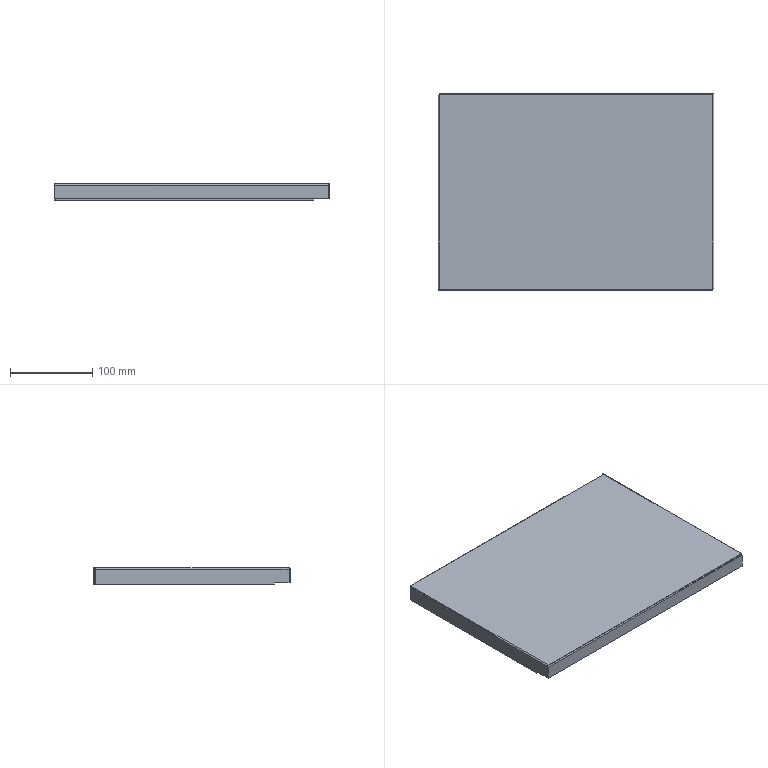Part | SolidWorks | features BaseBody 1 | 1 solid | 44 faces | box 336 x 239.8 x 20 mm | volume 120306 mm3 | plane 32 | cylinder 8 | spline 4 | commonest cylinder face diameters 1 x4 3.4 x4
STEP:
#1=CARTESIAN_POINT('',(-168.,-118.2,-18.));
#2=VERTEX_POINT('',#1);
#3=CARTESIAN_POINT('',(-168.,-100.2,-18.));
#4=VERTEX_POINT('',#3);
#5=CARTESIAN_POINT('',(-168.,-118.2,-18.));
#6=DIRECTION('',(0.,1.,0.));
#7=VECTOR('',#6,1000.);
#8=LINE('',#5,#7);
#9=EDGE_CURVE('',#2,#4,#8,.T.);
#10=ORIENTED_EDGE('',*,*,#9,.T.);
#11=CARTESIAN_POINT('',(-166.8,-100.2,-18.));
#12=VERTEX_POINT('',#11);
#13=CARTESIAN_POINT('',(-166.8,-100.2,-18.));
#14=DIRECTION('',(-1.,0.,0.));
#15=VECTOR('',#14,1000.);
#16=LINE('',#13,#15);
#17=EDGE_CURVE('',#12,#4,#16,.T.);
#18=ORIENTED_EDGE('',*,*,#17,.F.);
#19=CARTESIAN_POINT('',(-166.8,-118.2,-18.));
#20=VERTEX_POINT('',#19);
#21=CARTESIAN_POINT('',(-166.8,-118.2,-18.));
#22=DIRECTION('',(0.,1.,0.));
#23=VECTOR('',#22,1000.);
#24=LINE('',#21,#23);
#25=EDGE_CURVE('',#20,#12,#24,.T.);
#26=ORIENTED_EDGE('',*,*,#25,.F.);
#27=CARTESIAN_POINT('',(-166.8,-118.2,-18.));
#28=DIRECTION('',(-1.,0.,0.));
#29=VECTOR('',#28,1000.);
#30=LINE('',#27,#29);
#31=EDGE_CURVE('',#20,#2,#30,.T.);
#32=ORIENTED_EDGE('',*,*,#31,.T.);
#33=EDGE_LOOP('',(#10,#18,#26,#32));
#34=FACE_OUTER_BOUND('',#33,.T.);
#35=CARTESIAN_POINT('',(-166.8,-118.2,-18.));
#36=DIRECTION('',(0.,0.,1.));
#37=DIRECTION('',(1.,0.,0.));
#38=AXIS2_PLACEMENT_3D('',#35,#36,#37);
#39=PLANE('',#38);
#40=ADVANCED_FACE('',(#34),#39,.F.);
#41=CARTESIAN_POINT('',(-168.,-100.2,-20.));
#42=VERTEX_POINT('',#41);
#43=CARTESIAN_POINT('',(-168.,-100.2,-20.));
#44=DIRECTION('',(0.,0.,-1.));
#45=VECTOR('',#44,1000.);
#46=LINE('',#43,#45);
#47=EDGE_CURVE('',#4,#42,#46,.T.);
#48=ORIENTED_EDGE('',*,*,#47,.T.);
#49=CARTESIAN_POINT('',(-166.8,-100.2,-20.));
#50=VERTEX_POINT('',#49);
#51=CARTESIAN_POINT('',(-166.8,-100.2,-20.));
#52=DIRECTION('',(-1.,0.,0.));
#53=VECTOR('',#52,1000.);
#54=LINE('',#51,#53);
#55=EDGE_CURVE('',#50,#42,#54,.T.);
#56=ORIENTED_EDGE('',*,*,#55,.F.);
#57=CARTESIAN_POINT('',(-166.8,-100.2,-20.));
#58=DIRECTION('',(0.,0.,-1.));
#59=VECTOR('',#58,1000.);
#60=LINE('',#57,#59);
#61=EDGE_CURVE('',#12,#50,#60,.T.);
#62=ORIENTED_EDGE('',*,*,#61,.F.);
#63=ORIENTED_EDGE('',*,*,#17,.T.);
#64=EDGE_LOOP('',(#48,#56,#62,#63));
#65=FACE_OUTER_BOUND('',#64,.T.);
#66=CARTESIAN_POINT('',(-166.8,-100.2,-20.));
#67=DIRECTION('',(0.,1.,0.));
#68=DIRECTION('',(1.,0.,0.));
#69=AXIS2_PLACEMENT_3D('',#66,#67,#68);
#70=PLANE('',#69);
#71=ADVANCED_FACE('',(#65),#70,.F.);
#72=CARTESIAN_POINT('',(148.3,119.9,-20.));
#73=VERTEX_POINT('',#72);
#74=CARTESIAN_POINT('',(148.3,119.9,-18.));
#75=VERTEX_POINT('',#74);
#76=CARTESIAN_POINT('',(148.3,119.9,-20.));
#77=DIRECTION('',(0.,0.,1.));
#78=VECTOR('',#77,1000.);
#79=LINE('',#76,#78);
#80=EDGE_CURVE('',#73,#75,#79,.T.);
#81=ORIENTED_EDGE('',*,*,#80,.T.);
#82=CARTESIAN_POINT('',(148.3,118.7,-18.));
#83=VERTEX_POINT('',#82);
#84=CARTESIAN_POINT('',(148.3,118.7,-18.));
#85=DIRECTION('',(0.,1.,0.));
#86=VECTOR('',#85,1000.);
#87=LINE('',#84,#86);
#88=EDGE_CURVE('',#83,#75,#87,.T.);
#89=ORIENTED_EDGE('',*,*,#88,.F.);
#90=CARTESIAN_POINT('',(148.3,118.7,-20.));
#91=VERTEX_POINT('',#90);
#92=CARTESIAN_POINT('',(148.3,118.7,-20.));
#93=DIRECTION('',(0.,0.,1.));
#94=VECTOR('',#93,1000.);
#95=LINE('',#92,#94);
#96=EDGE_CURVE('',#91,#83,#95,.T.);
#97=ORIENTED_EDGE('',*,*,#96,.F.);
#98=CARTESIAN_POINT('',(148.3,118.7,-20.));
#99=DIRECTION('',(0.,1.,0.));
#100=VECTOR('',#99,1000.);
#101=LINE('',#98,#100);
#102=EDGE_CURVE('',#91,#73,#101,.T.);
#103=ORIENTED_EDGE('',*,*,#102,.T.);
#104=EDGE_LOOP('',(#81,#89,#97,#103));
#105=FACE_OUTER_BOUND('',#104,.T.);
#106=CARTESIAN_POINT('',(148.3,118.7,-20.));
#107=DIRECTION('',(-1.,0.,0.));
#108=DIRECTION('',(0.,1.,0.));
#109=AXIS2_PLACEMENT_3D('',#106,#107,#108);
#110=PLANE('',#109);
#111=ADVANCED_FACE('',(#105),#110,.F.);
#112=CARTESIAN_POINT('',(166.3,119.9,-18.));
#113=VERTEX_POINT('',#112);
#114=CARTESIAN_POINT('',(166.3,119.9,-18.));
#115=DIRECTION('',(1.,0.,0.));
#116=VECTOR('',#115,1000.);
#117=LINE('',#114,#116);
#118=EDGE_CURVE('',#75,#113,#117,.T.);
#119=ORIENTED_EDGE('',*,*,#118,.T.);
#120=CARTESIAN_POINT('',(166.3,118.7,-18.));
#121=VERTEX_POINT('',#120);
#122=CARTESIAN_POINT('',(166.3,118.7,-18.));
#123=DIRECTION('',(0.,1.,0.));
#124=VECTOR('',#123,1000.);
#125=LINE('',#122,#124);
#126=EDGE_CURVE('',#121,#113,#125,.T.);
#127=ORIENTED_EDGE('',*,*,#126,.F.);
#128=CARTESIAN_POINT('',(166.3,118.7,-18.));
#129=DIRECTION('',(1.,0.,0.));
#130=VECTOR('',#129,1000.);
#131=LINE('',#128,#130);
#132=EDGE_CURVE('',#83,#121,#131,.T.);
#133=ORIENTED_EDGE('',*,*,#132,.F.);
#134=ORIENTED_EDGE('',*,*,#88,.T.);
#135=EDGE_LOOP('',(#119,#127,#133,#134));
#136=FACE_OUTER_BOUND('',#135,.T.);
#137=CARTESIAN_POINT('',(166.3,118.7,-18.));
#138=DIRECTION('',(0.,0.,1.));
#139=DIRECTION('',(0.,-1.,0.));
#140=AXIS2_PLACEMENT_3D('',#137,#138,#139);
#141=PLANE('',#140);
#142=ADVANCED_FACE('',(#136),#141,.F.);
#143=CARTESIAN_POINT('',(166.3,118.7,-1.7));
#144=VERTEX_POINT('',#143);
#145=CARTESIAN_POINT('',(166.3,118.7,-20.));
#146=DIRECTION('',(0.,0.,-1.));
#147=VECTOR('',#146,1000.);
#148=LINE('',#145,#147);
#149=EDGE_CURVE('',#144,#121,#148,.T.);
#150=ORIENTED_EDGE('',*,*,#149,.T.);
#151=ORIENTED_EDGE('',*,*,#126,.T.);
#152=CARTESIAN_POINT('',(166.3,119.9,-1.7));
#153=VERTEX_POINT('',#152);
#154=CARTESIAN_POINT('',(166.3,119.9,0.));
#155=DIRECTION('',(0.,0.,-1.));
#156=VECTOR('',#155,1000.);
#157=LINE('',#154,#156);
#158=EDGE_CURVE('',#153,#113,#157,.T.);
#159=ORIENTED_EDGE('',*,*,#158,.F.);
#160=CARTESIAN_POINT('',(166.3,118.7,-1.7));
#161=DIRECTION('',(0.,1.,0.));
#162=VECTOR('',#161,1000.);
#163=LINE('',#160,#162);
#164=EDGE_CURVE('',#144,#153,#163,.T.);
#165=ORIENTED_EDGE('',*,*,#164,.F.);
#166=EDGE_LOOP('',(#150,#151,#159,#165));
#167=FACE_OUTER_BOUND('',#166,.T.);
#168=CARTESIAN_POINT('',(166.3,119.9,-20.));
#169=DIRECTION('',(-1.,0.,0.));
#170=DIRECTION('',(0.,1.,0.));
#171=AXIS2_PLACEMENT_3D('',#168,#169,#170);
#172=PLANE('',#171);
#173=ADVANCED_FACE('',(#167),#172,.F.);
#174=CARTESIAN_POINT('',(-166.093,119.9,-20.));
#175=VERTEX_POINT('',#174);
#176=CARTESIAN_POINT('',(0.,119.9,-20.));
#177=DIRECTION('',(-1.,0.,0.));
#178=VECTOR('',#177,1000.);
#179=LINE('',#176,#178);
#180=EDGE_CURVE('',#73,#175,#179,.T.);
#181=ORIENTED_EDGE('',*,*,#180,.F.);
#182=ORIENTED_EDGE('',*,*,#102,.F.);
#183=CARTESIAN_POINT('',(-166.093,118.7,-20.));
#184=VERTEX_POINT('',#183);
#185=CARTESIAN_POINT('',(-168.,118.7,-20.));
#186=DIRECTION('',(-1.,0.,0.));
#187=VECTOR('',#186,1000.);
#188=LINE('',#185,#187);
#189=EDGE_CURVE('',#91,#184,#188,.T.);
#190=ORIENTED_EDGE('',*,*,#189,.T.);
#191=CARTESIAN_POINT('',(-166.093,118.7,-20.));
#192=DIRECTION('',(0.,-1.,0.));
#193=VECTOR('',#192,1000.);
#194=LINE('',#191,#193);
#195=EDGE_CURVE('',#175,#184,#194,.T.);
#196=ORIENTED_EDGE('',*,*,#195,.F.);
#197=EDGE_LOOP('',(#181,#182,#190,#196));
#198=FACE_OUTER_BOUND('',#197,.T.);
#199=CARTESIAN_POINT('',(-168.,119.9,-20.));
#200=DIRECTION('',(0.,0.,1.));
#201=DIRECTION('',(0.,-1.,0.));
#202=AXIS2_PLACEMENT_3D('',#199,#200,#201);
#203=PLANE('',#202);
#204=ADVANCED_FACE('',(#198),#203,.F.);
#205=ORIENTED_EDGE('',*,*,#132,.T.);
#206=ORIENTED_EDGE('',*,*,#149,.F.);
#207=CARTESIAN_POINT('',(-166.093,118.7,-1.7));
#208=VERTEX_POINT('',#207);
#209=CARTESIAN_POINT('',(-168.,118.7,-1.7));
#210=DIRECTION('',(1.,0.,0.));
#211=VECTOR('',#210,1000.);
#212=LINE('',#209,#211);
#213=EDGE_CURVE('',#208,#144,#212,.T.);
#214=ORIENTED_EDGE('',*,*,#213,.F.);
#215=CARTESIAN_POINT('',(-166.093,118.7,0.));
#216=DIRECTION('',(0.,0.,-1.));
#217=VECTOR('',#216,1000.);
#218=LINE('',#215,#217);
#219=EDGE_CURVE('',#208,#184,#218,.T.);
#220=ORIENTED_EDGE('',*,*,#219,.T.);
#221=ORIENTED_EDGE('',*,*,#189,.F.);
#222=ORIENTED_EDGE('',*,*,#96,.T.);
#223=EDGE_LOOP('',(#205,#206,#214,#220,#221,#222));
#224=FACE_OUTER_BOUND('',#223,.T.);
#225=CARTESIAN_POINT('',(0.,118.7,0.));
#226=DIRECTION('',(0.,-1.,0.));
#227=DIRECTION('',(0.,0.,-1.));
#228=AXIS2_PLACEMENT_3D('',#225,#226,#227);
#229=PLANE('',#228);
#230=ADVANCED_FACE('',(#224),#229,.T.);
#231=ORIENTED_EDGE('',*,*,#158,.T.);
#232=ORIENTED_EDGE('',*,*,#118,.F.);
#233=ORIENTED_EDGE('',*,*,#80,.F.);
#234=ORIENTED_EDGE('',*,*,#180,.T.);
#235=CARTESIAN_POINT('',(-166.093,119.9,-1.7));
#236=VERTEX_POINT('',#235);
#237=CARTESIAN_POINT('',(-166.093,119.9,-1.2));
#238=DIRECTION('',(0.,0.,-1.));
#239=VECTOR('',#238,1000.);
#240=LINE('',#237,#239);
#241=EDGE_CURVE('',#236,#175,#240,.T.);
#242=ORIENTED_EDGE('',*,*,#241,.F.);
#243=CARTESIAN_POINT('',(-168.,119.9,-1.7));
#244=DIRECTION('',(-1.,0.,0.));
#245=VECTOR('',#244,1000.);
#246=LINE('',#243,#245);
#247=EDGE_CURVE('',#153,#236,#246,.T.);
#248=ORIENTED_EDGE('',*,*,#247,.F.);
#249=EDGE_LOOP('',(#231,#232,#233,#234,#242,#248));
#250=FACE_OUTER_BOUND('',#249,.T.);
#251=CARTESIAN_POINT('',(0.,119.9,0.));
#252=DIRECTION('',(0.,-1.,0.));
#253=DIRECTION('',(0.,0.,-1.));
#254=AXIS2_PLACEMENT_3D('',#251,#252,#253);
#255=PLANE('',#254);
#256=ADVANCED_FACE('',(#250),#255,.F.);
#257=ORIENTED_EDGE('',*,*,#241,.T.);
#258=ORIENTED_EDGE('',*,*,#195,.T.);
#259=ORIENTED_EDGE('',*,*,#219,.F.);
#260=CARTESIAN_POINT('',(-166.093,118.7,-1.7));
#261=DIRECTION('',(0.,-1.,0.));
#262=VECTOR('',#261,1000.);
#263=LINE('',#260,#262);
#264=EDGE_CURVE('',#236,#208,#263,.T.);
#265=ORIENTED_EDGE('',*,*,#264,.F.);
#266=EDGE_LOOP('',(#257,#258,#259,#265));
#267=FACE_OUTER_BOUND('',#266,.T.);
#268=CARTESIAN_POINT('',(-166.093,118.7,-1.2));
#269=DIRECTION('',(-1.,0.,0.));
#270=DIRECTION('',(0.,0.,1.));
#271=AXIS2_PLACEMENT_3D('',#268,#269,#270);
#272=PLANE('',#271);
#273=ADVANCED_FACE('',(#267),#272,.T.);
#274=CARTESIAN_POINT('',(166.3,118.2,-1.2));
#275=VERTEX_POINT('',#274);
#276=CARTESIAN_POINT('',(-166.3,118.2,-1.2));
#277=VERTEX_POINT('',#276);
#278=CARTESIAN_POINT('',(166.3,118.2,-1.2));
#279=DIRECTION('',(-1.,0.,0.));
#280=VECTOR('',#279,1000.);
#281=LINE('',#278,#280);
#282=EDGE_CURVE('',#275,#277,#281,.T.);
#283=ORIENTED_EDGE('',*,*,#282,.T.);
#284=CARTESIAN_POINT('',(-166.3,118.2,-1.2));
#285=CARTESIAN_POINT('',(-166.265,118.331,-1.2));
#286=CARTESIAN_POINT('',(-166.231,118.461,-1.254));
#287=CARTESIAN_POINT('',(-166.162,118.646,-1.439));
#288=CARTESIAN_POINT('',(-166.127,118.7,-1.569));
#289=CARTESIAN_POINT('',(-166.093,118.7,-1.7));
#290=B_SPLINE_CURVE_WITH_KNOTS('',3,(#284,#285,#286,#287,#288,#289),.UNSPECIFIED.,.F.,.F.,(4,2,4),(0.,0.5,1.),.UNSPECIFIED.);
#291=EDGE_CURVE('',#277,#208,#290,.T.);
#292=ORIENTED_EDGE('',*,*,#291,.T.);
#293=ORIENTED_EDGE('',*,*,#213,.T.);
#294=CARTESIAN_POINT('',(166.3,118.2,-1.7));
#295=DIRECTION('',(1.,0.,0.));
#296=DIRECTION('',(0.,0.,-1.));
#297=AXIS2_PLACEMENT_3D('',#294,#295,#296);
#298=CIRCLE('',#297,0.5);
#299=EDGE_CURVE('',#144,#275,#298,.T.);
#300=ORIENTED_EDGE('',*,*,#299,.T.);
#301=EDGE_LOOP('',(#283,#292,#293,#300));
#302=FACE_OUTER_BOUND('',#301,.T.);
#303=CARTESIAN_POINT('',(166.3,118.2,-1.7));
#304=DIRECTION('',(1.,0.,0.));
#305=DIRECTION('',(0.,1.,0.));
#306=AXIS2_PLACEMENT_3D('',#303,#304,#305);
#307=CYLINDRICAL_SURFACE('',#306,0.5);
#308=ADVANCED_FACE('',(#302),#307,.F.);
#309=CARTESIAN_POINT('',(166.3,118.2,0.));
#310=VERTEX_POINT('',#309);
#311=CARTESIAN_POINT('',(-166.3,118.2,0.));
#312=VERTEX_POINT('',#311);
#313=CARTESIAN_POINT('',(166.3,118.2,0.));
#314=DIRECTION('',(-1.,0.,0.));
#315=VECTOR('',#314,1000.);
#316=LINE('',#313,#315);
#317=EDGE_CURVE('',#310,#312,#316,.T.);
#318=ORIENTED_EDGE('',*,*,#317,.F.);
#319=CARTESIAN_POINT('',(166.3,119.825,-1.2));
#320=VERTEX_POINT('',#319);
#321=CARTESIAN_POINT('',(166.3,118.2,-1.7));
#322=DIRECTION('',(1.,0.,0.));
#323=DIRECTION('',(0.,0.,-1.));
#324=AXIS2_PLACEMENT_3D('',#321,#322,#323);
#325=CIRCLE('',#324,1.7);
#326=EDGE_CURVE('',#320,#310,#325,.T.);
#327=ORIENTED_EDGE('',*,*,#326,.F.);
#328=CARTESIAN_POINT('',(166.3,118.2,-1.7));
#329=DIRECTION('',(1.,0.,0.));
#330=DIRECTION('',(0.,0.,-1.));
#331=AXIS2_PLACEMENT_3D('',#328,#329,#330);
#332=CIRCLE('',#331,1.7);
#333=EDGE_CURVE('',#153,#320,#332,.T.);
#334=ORIENTED_EDGE('',*,*,#333,.F.);
#335=ORIENTED_EDGE('',*,*,#247,.T.);
#336=CARTESIAN_POINT('',(-166.3,118.2,0.));
#337=CARTESIAN_POINT('',(-166.283,118.423,0.));
#338=CARTESIAN_POINT('',(-166.265,118.645,-0.04425));
#339=CARTESIAN_POINT('',(-166.231,119.056,-0.2146));
#340=CARTESIAN_POINT('',(-166.214,119.245,-0.3406));
#341=CARTESIAN_POINT('',(-166.179,119.559,-0.6553));
#342=CARTESIAN_POINT('',(-166.162,119.685,-0.8438));
#343=CARTESIAN_POINT('',(-166.127,119.856,-1.255));
#344=CARTESIAN_POINT('',(-166.11,119.9,-1.477));
#345=CARTESIAN_POINT('',(-166.093,119.9,-1.7));
#346=B_SPLINE_CURVE_WITH_KNOTS('',3,(#336,#337,#338,#339,#340,#341,#342,#343,#344,#345),.UNSPECIFIED.,.F.,.F.,(4,2,2,2,4),(0.,0.25,0.5,0.75,1.),.UNSPECIFIED.);
#347=EDGE_CURVE('',#312,#236,#346,.T.);
#348=ORIENTED_EDGE('',*,*,#347,.F.);
#349=EDGE_LOOP('',(#318,#327,#334,#335,#348));
#350=FACE_OUTER_BOUND('',#349,.T.);
#351=CARTESIAN_POINT('',(166.3,118.2,-1.7));
#352=DIRECTION('',(1.,0.,0.));
#353=DIRECTION('',(0.,1.,0.));
#354=AXIS2_PLACEMENT_3D('',#351,#352,#353);
#355=CYLINDRICAL_SURFACE('',#354,1.7);
#356=ADVANCED_FACE('',(#350),#355,.T.);
#357=ORIENTED_EDGE('',*,*,#333,.T.);
#358=CARTESIAN_POINT('',(166.3,119.9,-1.2));
#359=DIRECTION('',(0.,-1.,0.));
#360=VECTOR('',#359,1000.);
#361=LINE('',#358,#360);
#362=EDGE_CURVE('',#320,#275,#361,.T.);
#363=ORIENTED_EDGE('',*,*,#362,.T.);
#364=ORIENTED_EDGE('',*,*,#299,.F.);
#365=ORIENTED_EDGE('',*,*,#164,.T.);
#366=EDGE_LOOP('',(#357,#363,#364,#365));
#367=FACE_OUTER_BOUND('',#366,.T.);
#368=CARTESIAN_POINT('',(166.3,118.2,-1.7));
#369=DIRECTION('',(-1.,0.,0.));
#370=DIRECTION('',(0.,1.,0.));
#371=AXIS2_PLACEMENT_3D('',#368,#369,#370);
#372=PLANE('',#371);
#373=ADVANCED_FACE('',(#367),#372,.F.);
#374=ORIENTED_EDGE('',*,*,#264,.T.);
#375=ORIENTED_EDGE('',*,*,#291,.F.);
#376=CARTESIAN_POINT('',(-166.3,118.2,-1.2));
#377=DIRECTION('',(0.,0.,1.));
#378=VECTOR('',#377,1000.);
#379=LINE('',#376,#378);
#380=EDGE_CURVE('',#277,#312,#379,.T.);
#381=ORIENTED_EDGE('',*,*,#380,.T.);
#382=ORIENTED_EDGE('',*,*,#347,.T.);
#383=EDGE_LOOP('',(#374,#375,#381,#382));
#384=FACE_OUTER_BOUND('',#383,.T.);
#385=CARTESIAN_POINT('',(-166.3,118.2,0.012));
#386=CARTESIAN_POINT('',(-166.283,118.424,0.012));
#387=CARTESIAN_POINT('',(-166.265,118.648,-0.03256));
#388=CARTESIAN_POINT('',(-166.231,119.062,-0.2041));
#389=CARTESIAN_POINT('',(-166.214,119.252,-0.331));
#390=CARTESIAN_POINT('',(-166.179,119.569,-0.6479));
#391=CARTESIAN_POINT('',(-166.162,119.696,-0.8378));
#392=CARTESIAN_POINT('',(-166.127,119.867,-1.252));
#393=CARTESIAN_POINT('',(-166.11,119.912,-1.476));
#394=CARTESIAN_POINT('',(-166.093,119.912,-1.7));
#395=CARTESIAN_POINT('',(-166.3,118.2,0.));
#396=CARTESIAN_POINT('',(-166.283,118.423,0.));
#397=CARTESIAN_POINT('',(-166.265,118.645,-0.04425));
#398=CARTESIAN_POINT('',(-166.231,119.056,-0.2146));
#399=CARTESIAN_POINT('',(-166.214,119.245,-0.3406));
#400=CARTESIAN_POINT('',(-166.179,119.559,-0.6553));
#401=CARTESIAN_POINT('',(-166.162,119.685,-0.8438));
#402=CARTESIAN_POINT('',(-166.127,119.856,-1.255));
#403=CARTESIAN_POINT('',(-166.11,119.9,-1.477));
#404=CARTESIAN_POINT('',(-166.093,119.9,-1.7));
#405=CARTESIAN_POINT('',(-166.3,118.2,-1.2));
#406=CARTESIAN_POINT('',(-166.283,118.265,-1.2));
#407=CARTESIAN_POINT('',(-166.265,118.331,-1.213));
#408=CARTESIAN_POINT('',(-166.231,118.452,-1.263));
#409=CARTESIAN_POINT('',(-166.214,118.507,-1.3));
#410=CARTESIAN_POINT('',(-166.179,118.6,-1.393));
#411=CARTESIAN_POINT('',(-166.162,118.637,-1.448));
#412=CARTESIAN_POINT('',(-166.127,118.687,-1.569));
#413=CARTESIAN_POINT('',(-166.11,118.7,-1.635));
#414=CARTESIAN_POINT('',(-166.093,118.7,-1.7));
#415=CARTESIAN_POINT('',(-166.3,118.2,-1.212));
#416=CARTESIAN_POINT('',(-166.283,118.264,-1.212));
#417=CARTESIAN_POINT('',(-166.265,118.328,-1.225));
#418=CARTESIAN_POINT('',(-166.231,118.446,-1.274));
#419=CARTESIAN_POINT('',(-166.214,118.5,-1.31));
#420=CARTESIAN_POINT('',(-166.179,118.59,-1.4));
#421=CARTESIAN_POINT('',(-166.162,118.626,-1.454));
#422=CARTESIAN_POINT('',(-166.127,118.675,-1.572));
#423=CARTESIAN_POINT('',(-166.11,118.688,-1.636));
#424=CARTESIAN_POINT('',(-166.093,118.688,-1.7));
#425=B_SPLINE_SURFACE_WITH_KNOTS('',1,3,((#385,#386,#387,#388,#389,#390,#391,#392,#393,#394),(#395,#396,#397,#398,#399,#400,#401,#402,#403,#404),(#405,#406,#407,#408,#409,#410,#411,#412,#413,#414),(#415,#416,#417,#418,#419,#420,#421,#422,#423,#424)),.UNSPECIFIED.,.F.,.F.,.F.,(2,1,1,2),(4,2,2,2,4),(-0.01,0.,1.,1.01),(0.,0.25,0.5,0.75,1.),.UNSPECIFIED.);
#426=ADVANCED_FACE('',(#384),#425,.F.);
#427=CARTESIAN_POINT('',(-168.,117.993,-20.));
#428=VERTEX_POINT('',#427);
#429=CARTESIAN_POINT('',(-166.8,117.993,-20.));
#430=VERTEX_POINT('',#429);
#431=CARTESIAN_POINT('',(-168.,117.993,-20.));
#432=DIRECTION('',(1.,0.,0.));
#433=VECTOR('',#432,1000.);
#434=LINE('',#431,#433);
#435=EDGE_CURVE('',#428,#430,#434,.T.);
#436=ORIENTED_EDGE('',*,*,#435,.F.);
#437=CARTESIAN_POINT('',(-168.,117.993,-1.7));
#438=VERTEX_POINT('',#437);
#439=CARTESIAN_POINT('',(-168.,117.993,0.));
#440=DIRECTION('',(0.,0.,-1.));
#441=VECTOR('',#440,1000.);
#442=LINE('',#439,#441);
#443=EDGE_CURVE('',#438,#428,#442,.T.);
#444=ORIENTED_EDGE('',*,*,#443,.F.);
#445=CARTESIAN_POINT('',(-166.8,117.993,-1.7));
#446=VERTEX_POINT('',#445);
#447=CARTESIAN_POINT('',(-166.8,117.993,-1.7));
#448=DIRECTION('',(1.,0.,0.));
#449=VECTOR('',#448,1000.);
#450=LINE('',#447,#449);
#451=EDGE_CURVE('',#438,#446,#450,.T.);
#452=ORIENTED_EDGE('',*,*,#451,.T.);
#453=CARTESIAN_POINT('',(-166.8,117.993,-1.2));
#454=DIRECTION('',(0.,0.,-1.));
#455=VECTOR('',#454,1000.);
#456=LINE('',#453,#455);
#457=EDGE_CURVE('',#446,#430,#456,.T.);
#458=ORIENTED_EDGE('',*,*,#457,.T.);
#459=EDGE_LOOP('',(#436,#444,#452,#458));
#460=FACE_OUTER_BOUND('',#459,.T.);
#461=CARTESIAN_POINT('',(-166.8,117.993,-1.2));
#462=DIRECTION('',(0.,-1.,0.));
#463=DIRECTION('',(0.,0.,-1.));
#464=AXIS2_PLACEMENT_3D('',#461,#462,#463);
#465=PLANE('',#464);
#466=ADVANCED_FACE('',(#460),#465,.F.);
#467=CARTESIAN_POINT('',(-166.8,-118.2,-20.));
#468=DIRECTION('',(0.,-1.,0.));
#469=VECTOR('',#468,1000.);
#470=LINE('',#467,#469);
#471=EDGE_CURVE('',#430,#50,#470,.T.);
#472=ORIENTED_EDGE('',*,*,#471,.T.);
#473=ORIENTED_EDGE('',*,*,#55,.T.);
#474=CARTESIAN_POINT('',(-168.,0.,-20.));
#475=DIRECTION('',(0.,-1.,0.));
#476=VECTOR('',#475,1000.);
#477=LINE('',#474,#476);
#478=EDGE_CURVE('',#428,#42,#477,.T.);
#479=ORIENTED_EDGE('',*,*,#478,.F.);
#480=ORIENTED_EDGE('',*,*,#435,.T.);
#481=EDGE_LOOP('',(#472,#473,#479,#480));
#482=FACE_OUTER_BOUND('',#481,.T.);
#483=CARTESIAN_POINT('',(-168.,-118.2,-20.));
#484=DIRECTION('',(0.,0.,1.));
#485=DIRECTION('',(1.,0.,0.));
#486=AXIS2_PLACEMENT_3D('',#483,#484,#485);
#487=PLANE('',#486);
#488=ADVANCED_FACE('',(#482),#487,.F.);
#489=ORIENTED_EDGE('',*,*,#61,.T.);
#490=ORIENTED_EDGE('',*,*,#471,.F.);
#491=ORIENTED_EDGE('',*,*,#457,.F.);
#492=CARTESIAN_POINT('',(-166.8,-118.2,-1.7));
#493=VERTEX_POINT('',#492);
#494=CARTESIAN_POINT('',(-166.8,-118.2,-1.7));
#495=DIRECTION('',(0.,1.,0.));
#496=VECTOR('',#495,1000.);
#497=LINE('',#494,#496);
#498=EDGE_CURVE('',#493,#446,#497,.T.);
#499=ORIENTED_EDGE('',*,*,#498,.F.);
#500=CARTESIAN_POINT('',(-166.8,-118.2,-1.2));
#501=DIRECTION('',(0.,0.,1.));
#502=VECTOR('',#501,1000.);
#503=LINE('',#500,#502);
#504=EDGE_CURVE('',#20,#493,#503,.T.);
#505=ORIENTED_EDGE('',*,*,#504,.F.);
#506=ORIENTED_EDGE('',*,*,#25,.T.);
#507=EDGE_LOOP('',(#489,#490,#491,#499,#505,#506));
#508=FACE_OUTER_BOUND('',#507,.T.);
#509=CARTESIAN_POINT('',(-166.8,0.,0.));
#510=DIRECTION('',(1.,0.,0.));
#511=DIRECTION('',(0.,0.,-1.));
#512=AXIS2_PLACEMENT_3D('',#509,#510,#511);
#513=PLANE('',#512);
#514=ADVANCED_FACE('',(#508),#513,.T.);
#515=ORIENTED_EDGE('',*,*,#478,.T.);
#516=ORIENTED_EDGE('',*,*,#47,.F.);
#517=ORIENTED_EDGE('',*,*,#9,.F.);
#518=CARTESIAN_POINT('',(-168.,-118.2,-1.7));
#519=VERTEX_POINT('',#518);
#520=CARTESIAN_POINT('',(-168.,-118.2,0.));
#521=DIRECTION('',(0.,0.,1.));
#522=VECTOR('',#521,1000.);
#523=LINE('',#520,#522);
#524=EDGE_CURVE('',#2,#519,#523,.T.);
#525=ORIENTED_EDGE('',*,*,#524,.T.);
#526=CARTESIAN_POINT('',(-168.,-118.2,-1.7));
#527=DIRECTION('',(0.,-1.,0.));
#528=VECTOR('',#527,1000.);
#529=LINE('',#526,#528);
#530=EDGE_CURVE('',#438,#519,#529,.T.);
#531=ORIENTED_EDGE('',*,*,#530,.F.);
#532=ORIENTED_EDGE('',*,*,#443,.T.);
#533=EDGE_LOOP('',(#515,#516,#517,#525,#531,#532));
#534=FACE_OUTER_BOUND('',#533,.T.);
#535=CARTESIAN_POINT('',(-168.,0.,0.));
#536=DIRECTION('',(1.,0.,0.));
#537=DIRECTION('',(0.,0.,-1.));
#538=AXIS2_PLACEMENT_3D('',#535,#536,#537);
#539=PLANE('',#538);
#540=ADVANCED_FACE('',(#534),#539,.F.);
#541=ORIENTED_EDGE('',*,*,#524,.F.);
#542=ORIENTED_EDGE('',*,*,#31,.F.);
#543=ORIENTED_EDGE('',*,*,#504,.T.);
#544=CARTESIAN_POINT('',(-168.,-118.2,-1.7));
#545=DIRECTION('',(-1.,0.,0.));
#546=VECTOR('',#545,1000.);
#547=LINE('',#544,#546);
#548=EDGE_CURVE('',#493,#519,#547,.T.);
#549=ORIENTED_EDGE('',*,*,#548,.T.);
#550=EDGE_LOOP('',(#541,#542,#543,#549));
#551=FACE_OUTER_BOUND('',#550,.T.);
#552=CARTESIAN_POINT('',(-168.,-118.2,-1.2));
#553=DIRECTION('',(0.,1.,0.));
#554=DIRECTION('',(1.,0.,0.));
#555=AXIS2_PLACEMENT_3D('',#552,#553,#554);
#556=PLANE('',#555);
#557=ADVANCED_FACE('',(#551),#556,.F.);
#558=CARTESIAN_POINT('',(-166.3,-118.2,-1.2));
#559=VERTEX_POINT('',#558);
#560=CARTESIAN_POINT('',(-166.3,118.2,-1.2));
#561=DIRECTION('',(0.,-1.,0.));
#562=VECTOR('',#561,1000.);
#563=LINE('',#560,#562);
#564=EDGE_CURVE('',#277,#559,#563,.T.);
#565=ORIENTED_EDGE('',*,*,#564,.T.);
#566=CARTESIAN_POINT('',(-166.3,-118.2,-1.7));
#567=DIRECTION('',(0.,-1.,0.));
#568=DIRECTION('',(0.,0.,1.));
#569=AXIS2_PLACEMENT_3D('',#566,#567,#568);
#570=CIRCLE('',#569,0.5);
#571=EDGE_CURVE('',#559,#493,#570,.T.);
#572=ORIENTED_EDGE('',*,*,#571,.T.);
#573=ORIENTED_EDGE('',*,*,#498,.T.);
#574=CARTESIAN_POINT('',(-166.8,117.993,-1.7));
#575=CARTESIAN_POINT('',(-166.8,118.027,-1.569));
#576=CARTESIAN_POINT('',(-166.746,118.062,-1.439));
#577=CARTESIAN_POINT('',(-166.561,118.131,-1.254));
#578=CARTESIAN_POINT('',(-166.431,118.165,-1.2));
#579=CARTESIAN_POINT('',(-166.3,118.2,-1.2));
#580=B_SPLINE_CURVE_WITH_KNOTS('',3,(#574,#575,#576,#577,#578,#579),.UNSPECIFIED.,.F.,.F.,(4,2,4),(0.,0.5,1.),.UNSPECIFIED.);
#581=EDGE_CURVE('',#446,#277,#580,.T.);
#582=ORIENTED_EDGE('',*,*,#581,.T.);
#583=EDGE_LOOP('',(#565,#572,#573,#582));
#584=FACE_OUTER_BOUND('',#583,.T.);
#585=CARTESIAN_POINT('',(-166.3,118.2,-1.7));
#586=DIRECTION('',(0.,1.,0.));
#587=DIRECTION('',(-1.,0.,0.));
#588=AXIS2_PLACEMENT_3D('',#585,#586,#587);
#589=CYLINDRICAL_SURFACE('',#588,0.5);
#590=ADVANCED_FACE('',(#584),#589,.F.);
#591=CARTESIAN_POINT('',(-166.3,-118.2,0.));
#592=VERTEX_POINT('',#591);
#593=CARTESIAN_POINT('',(-166.3,118.2,0.));
#594=DIRECTION('',(0.,-1.,0.));
#595=VECTOR('',#594,1000.);
#596=LINE('',#593,#595);
#597=EDGE_CURVE('',#312,#592,#596,.T.);
#598=ORIENTED_EDGE('',*,*,#597,.F.);
#599=CARTESIAN_POINT('',(-168.,117.993,-1.7));
#600=CARTESIAN_POINT('',(-168.,118.01,-1.477));
#601=CARTESIAN_POINT('',(-167.956,118.027,-1.255));
#602=CARTESIAN_POINT('',(-167.785,118.062,-0.8438));
#603=CARTESIAN_POINT('',(-167.659,118.079,-0.6553));
#604=CARTESIAN_POINT('',(-167.345,118.114,-0.3406));
#605=CARTESIAN_POINT('',(-167.156,118.131,-0.2146));
#606=CARTESIAN_POINT('',(-166.745,118.165,-0.04425));
#607=CARTESIAN_POINT('',(-166.523,118.183,0.));
#608=CARTESIAN_POINT('',(-166.3,118.2,0.));
#609=B_SPLINE_CURVE_WITH_KNOTS('',3,(#599,#600,#601,#602,#603,#604,#605,#606,#607,#608),.UNSPECIFIED.,.F.,.F.,(4,2,2,2,4),(0.,0.25,0.5,0.75,1.),.UNSPECIFIED.);
#610=EDGE_CURVE('',#438,#312,#609,.T.);
#611=ORIENTED_EDGE('',*,*,#610,.F.);
#612=ORIENTED_EDGE('',*,*,#530,.T.);
#613=CARTESIAN_POINT('',(-167.925,-118.2,-1.2));
#614=VERTEX_POINT('',#613);
#615=CARTESIAN_POINT('',(-166.3,-118.2,-1.7));
#616=DIRECTION('',(0.,-1.,0.));
#617=DIRECTION('',(0.,0.,1.));
#618=AXIS2_PLACEMENT_3D('',#615,#616,#617);
#619=CIRCLE('',#618,1.7);
#620=EDGE_CURVE('',#614,#519,#619,.T.);
#621=ORIENTED_EDGE('',*,*,#620,.F.);
#622=CARTESIAN_POINT('',(-166.3,-118.2,-1.7));
#623=DIRECTION('',(0.,-1.,0.));
#624=DIRECTION('',(0.,0.,1.));
#625=AXIS2_PLACEMENT_3D('',#622,#623,#624);
#626=CIRCLE('',#625,1.7);
#627=EDGE_CURVE('',#592,#614,#626,.T.);
#628=ORIENTED_EDGE('',*,*,#627,.F.);
#629=EDGE_LOOP('',(#598,#611,#612,#621,#628));
#630=FACE_OUTER_BOUND('',#629,.T.);
#631=CARTESIAN_POINT('',(-166.3,118.2,-1.7));
#632=DIRECTION('',(0.,1.,0.));
#633=DIRECTION('',(-1.,0.,0.));
#634=AXIS2_PLACEMENT_3D('',#631,#632,#633);
#635=CYLINDRICAL_SURFACE('',#634,1.7);
#636=ADVANCED_FACE('',(#630),#635,.T.);
#637=ORIENTED_EDGE('',*,*,#581,.F.);
#638=ORIENTED_EDGE('',*,*,#451,.F.);
#639=ORIENTED_EDGE('',*,*,#610,.T.);
#640=ORIENTED_EDGE('',*,*,#380,.F.);
#641=EDGE_LOOP('',(#637,#638,#639,#640));
#642=FACE_OUTER_BOUND('',#641,.T.);
#643=CARTESIAN_POINT('',(-168.012,117.993,-1.7));
#644=CARTESIAN_POINT('',(-168.012,118.01,-1.476));
#645=CARTESIAN_POINT('',(-167.967,118.027,-1.252));
#646=CARTESIAN_POINT('',(-167.796,118.062,-0.8378));
#647=CARTESIAN_POINT('',(-167.669,118.079,-0.6479));
#648=CARTESIAN_POINT('',(-167.352,118.114,-0.331));
#649=CARTESIAN_POINT('',(-167.162,118.131,-0.2041));
#650=CARTESIAN_POINT('',(-166.748,118.165,-0.03256));
#651=CARTESIAN_POINT('',(-166.524,118.183,0.012));
#652=CARTESIAN_POINT('',(-166.3,118.2,0.012));
#653=CARTESIAN_POINT('',(-168.,117.993,-1.7));
#654=CARTESIAN_POINT('',(-168.,118.01,-1.477));
#655=CARTESIAN_POINT('',(-167.956,118.027,-1.255));
#656=CARTESIAN_POINT('',(-167.785,118.062,-0.8438));
#657=CARTESIAN_POINT('',(-167.659,118.079,-0.6553));
#658=CARTESIAN_POINT('',(-167.345,118.114,-0.3406));
#659=CARTESIAN_POINT('',(-167.156,118.131,-0.2146));
#660=CARTESIAN_POINT('',(-166.745,118.165,-0.04425));
#661=CARTESIAN_POINT('',(-166.523,118.183,0.));
#662=CARTESIAN_POINT('',(-166.3,118.2,0.));
#663=CARTESIAN_POINT('',(-166.8,117.993,-1.7));
#664=CARTESIAN_POINT('',(-166.8,118.01,-1.635));
#665=CARTESIAN_POINT('',(-166.787,118.027,-1.569));
#666=CARTESIAN_POINT('',(-166.737,118.062,-1.448));
#667=CARTESIAN_POINT('',(-166.7,118.079,-1.393));
#668=CARTESIAN_POINT('',(-166.607,118.114,-1.3));
#669=CARTESIAN_POINT('',(-166.552,118.131,-1.263));
#670=CARTESIAN_POINT('',(-166.431,118.165,-1.213));
#671=CARTESIAN_POINT('',(-166.365,118.183,-1.2));
#672=CARTESIAN_POINT('',(-166.3,118.2,-1.2));
#673=CARTESIAN_POINT('',(-166.788,117.993,-1.7));
#674=CARTESIAN_POINT('',(-166.788,118.01,-1.636));
#675=CARTESIAN_POINT('',(-166.775,118.027,-1.572));
#676=CARTESIAN_POINT('',(-166.726,118.062,-1.454));
#677=CARTESIAN_POINT('',(-166.69,118.079,-1.4));
#678=CARTESIAN_POINT('',(-166.6,118.114,-1.31));
#679=CARTESIAN_POINT('',(-166.546,118.131,-1.274));
#680=CARTESIAN_POINT('',(-166.428,118.165,-1.225));
#681=CARTESIAN_POINT('',(-166.364,118.183,-1.212));
#682=CARTESIAN_POINT('',(-166.3,118.2,-1.212));
#683=B_SPLINE_SURFACE_WITH_KNOTS('',1,3,((#643,#644,#645,#646,#647,#648,#649,#650,#651,#652),(#653,#654,#655,#656,#657,#658,#659,#660,#661,#662),(#663,#664,#665,#666,#667,#668,#669,#670,#671,#672),(#673,#674,#675,#676,#677,#678,#679,#680,#681,#682)),.UNSPECIFIED.,.F.,.F.,.F.,(2,1,1,2),(4,2,2,2,4),(-0.01,0.,1.,1.01),(0.,0.25,0.5,0.75,1.),.UNSPECIFIED.);
#684=ADVANCED_FACE('',(#642),#683,.F.);
#685=CARTESIAN_POINT('',(-168.,-118.2,-1.2));
#686=DIRECTION('',(1.,0.,0.));
#687=VECTOR('',#686,1000.);
#688=LINE('',#685,#687);
#689=EDGE_CURVE('',#614,#559,#688,.T.);
#690=ORIENTED_EDGE('',*,*,#689,.F.);
#691=ORIENTED_EDGE('',*,*,#620,.T.);
#692=ORIENTED_EDGE('',*,*,#548,.F.);
#693=ORIENTED_EDGE('',*,*,#571,.F.);
#694=EDGE_LOOP('',(#690,#691,#692,#693));
#695=FACE_OUTER_BOUND('',#694,.T.);
#696=CARTESIAN_POINT('',(-166.3,-118.2,-1.7));
#697=DIRECTION('',(0.,-1.,0.));
#698=DIRECTION('',(0.,0.,-1.));
#699=AXIS2_PLACEMENT_3D('',#696,#697,#698);
#700=PLANE('',#699);
#701=ADVANCED_FACE('',(#695),#700,.T.);
#702=CARTESIAN_POINT('',(168.,-117.993,-18.));
#703=VERTEX_POINT('',#702);
#704=CARTESIAN_POINT('',(166.8,-117.993,-18.));
#705=VERTEX_POINT('',#704);
#706=CARTESIAN_POINT('',(168.,-117.993,-18.));
#707=DIRECTION('',(-1.,0.,0.));
#708=VECTOR('',#707,1000.);
#709=LINE('',#706,#708);
#710=EDGE_CURVE('',#703,#705,#709,.T.);
#711=ORIENTED_EDGE('',*,*,#710,.F.);
#712=CARTESIAN_POINT('',(168.,-117.993,-1.7));
#713=VERTEX_POINT('',#712);
#714=CARTESIAN_POINT('',(168.,-117.993,0.));
#715=DIRECTION('',(0.,0.,-1.));
#716=VECTOR('',#715,1000.);
#717=LINE('',#714,#716);
#718=EDGE_CURVE('',#713,#703,#717,.T.);
#719=ORIENTED_EDGE('',*,*,#718,.F.);
#720=CARTESIAN_POINT('',(166.8,-117.993,-1.7));
#721=VERTEX_POINT('',#720);
#722=CARTESIAN_POINT('',(166.8,-117.993,-1.7));
#723=DIRECTION('',(-1.,0.,0.));
#724=VECTOR('',#723,1000.);
#725=LINE('',#722,#724);
#726=EDGE_CURVE('',#713,#721,#725,.T.);
#727=ORIENTED_EDGE('',*,*,#726,.T.);
#728=CARTESIAN_POINT('',(166.8,-117.993,-1.2));
#729=DIRECTION('',(0.,0.,-1.));
#730=VECTOR('',#729,1000.);
#731=LINE('',#728,#730);
#732=EDGE_CURVE('',#721,#705,#731,.T.);
#733=ORIENTED_EDGE('',*,*,#732,.T.);
#734=EDGE_LOOP('',(#711,#719,#727,#733));
#735=FACE_OUTER_BOUND('',#734,.T.);
#736=CARTESIAN_POINT('',(166.8,-117.993,-1.2));
#737=DIRECTION('',(0.,1.,0.));
#738=DIRECTION('',(0.,0.,-1.));
#739=AXIS2_PLACEMENT_3D('',#736,#737,#738);
#740=PLANE('',#739);
#741=ADVANCED_FACE('',(#735),#740,.F.);
#742=CARTESIAN_POINT('',(168.,119.9,-18.));
#743=VERTEX_POINT('',#742);
#744=CARTESIAN_POINT('',(168.,0.,-18.));
#745=DIRECTION('',(0.,1.,0.));
#746=VECTOR('',#745,1000.);
#747=LINE('',#744,#746);
#748=EDGE_CURVE('',#703,#743,#747,.T.);
#749=ORIENTED_EDGE('',*,*,#748,.F.);
#750=ORIENTED_EDGE('',*,*,#710,.T.);
#751=CARTESIAN_POINT('',(166.8,119.9,-18.));
#752=VERTEX_POINT('',#751);
#753=CARTESIAN_POINT('',(166.8,119.9,-18.));
#754=DIRECTION('',(0.,1.,0.));
#755=VECTOR('',#754,1000.);
#756=LINE('',#753,#755);
#757=EDGE_CURVE('',#705,#752,#756,.T.);
#758=ORIENTED_EDGE('',*,*,#757,.T.);
#759=CARTESIAN_POINT('',(168.,119.9,-18.));
#760=DIRECTION('',(-1.,0.,0.));
#761=VECTOR('',#760,1000.);
#762=LINE('',#759,#761);
#763=EDGE_CURVE('',#743,#752,#762,.T.);
#764=ORIENTED_EDGE('',*,*,#763,.F.);
#765=EDGE_LOOP('',(#749,#750,#758,#764));
#766=FACE_OUTER_BOUND('',#765,.T.);
#767=CARTESIAN_POINT('',(168.,119.9,-18.));
#768=DIRECTION('',(0.,0.,1.));
#769=DIRECTION('',(1.,0.,0.));
#770=AXIS2_PLACEMENT_3D('',#767,#768,#769);
#771=PLANE('',#770);
#772=ADVANCED_FACE('',(#766),#771,.F.);
#773=ORIENTED_EDGE('',*,*,#732,.F.);
#774=CARTESIAN_POINT('',(166.8,119.9,-1.7));
#775=VERTEX_POINT('',#774);
#776=CARTESIAN_POINT('',(166.8,119.9,-1.7));
#777=DIRECTION('',(0.,-1.,0.));
#778=VECTOR('',#777,1000.);
#779=LINE('',#776,#778);
#780=EDGE_CURVE('',#775,#721,#779,.T.);
#781=ORIENTED_EDGE('',*,*,#780,.F.);
#782=CARTESIAN_POINT('',(166.8,119.9,-1.2));
#783=DIRECTION('',(0.,0.,1.));
#784=VECTOR('',#783,1000.);
#785=LINE('',#782,#784);
#786=EDGE_CURVE('',#752,#775,#785,.T.);
#787=ORIENTED_EDGE('',*,*,#786,.F.);
#788=ORIENTED_EDGE('',*,*,#757,.F.);
#789=EDGE_LOOP('',(#773,#781,#787,#788));
#790=FACE_OUTER_BOUND('',#789,.T.);
#791=CARTESIAN_POINT('',(166.8,0.,0.));
#792=DIRECTION('',(-1.,0.,0.));
#793=DIRECTION('',(0.,0.,1.));
#794=AXIS2_PLACEMENT_3D('',#791,#792,#793);
#795=PLANE('',#794);
#796=ADVANCED_FACE('',(#790),#795,.T.);
#797=CARTESIAN_POINT('',(168.,119.9,-1.7));
#798=VERTEX_POINT('',#797);
#799=CARTESIAN_POINT('',(168.,119.9,-1.7));
#800=DIRECTION('',(0.,1.,0.));
#801=VECTOR('',#800,1000.);
#802=LINE('',#799,#801);
#803=EDGE_CURVE('',#713,#798,#802,.T.);
#804=ORIENTED_EDGE('',*,*,#803,.F.);
#805=ORIENTED_EDGE('',*,*,#718,.T.);
#806=ORIENTED_EDGE('',*,*,#748,.T.);
#807=CARTESIAN_POINT('',(168.,119.9,0.));
#808=DIRECTION('',(0.,0.,1.));
#809=VECTOR('',#808,1000.);
#810=LINE('',#807,#809);
#811=EDGE_CURVE('',#743,#798,#810,.T.);
#812=ORIENTED_EDGE('',*,*,#811,.T.);
#813=EDGE_LOOP('',(#804,#805,#806,#812));
#814=FACE_OUTER_BOUND('',#813,.T.);
#815=CARTESIAN_POINT('',(168.,0.,0.));
#816=DIRECTION('',(-1.,0.,0.));
#817=DIRECTION('',(0.,0.,1.));
#818=AXIS2_PLACEMENT_3D('',#815,#816,#817);
#819=PLANE('',#818);
#820=ADVANCED_FACE('',(#814),#819,.F.);
#821=CARTESIAN_POINT('',(168.,119.9,-1.7));
#822=DIRECTION('',(1.,0.,0.));
#823=VECTOR('',#822,1000.);
#824=LINE('',#821,#823);
#825=EDGE_CURVE('',#775,#798,#824,.T.);
#826=ORIENTED_EDGE('',*,*,#825,.T.);
#827=ORIENTED_EDGE('',*,*,#811,.F.);
#828=ORIENTED_EDGE('',*,*,#763,.T.);
#829=ORIENTED_EDGE('',*,*,#786,.T.);
#830=EDGE_LOOP('',(#826,#827,#828,#829));
#831=FACE_OUTER_BOUND('',#830,.T.);
#832=CARTESIAN_POINT('',(168.,119.9,-1.2));
#833=DIRECTION('',(0.,-1.,0.));
#834=DIRECTION('',(0.,0.,-1.));
#835=AXIS2_PLACEMENT_3D('',#832,#833,#834);
#836=PLANE('',#835);
#837=ADVANCED_FACE('',(#831),#836,.F.);
#838=CARTESIAN_POINT('',(166.3,-118.2,-1.2));
#839=VERTEX_POINT('',#838);
#840=CARTESIAN_POINT('',(166.3,-118.2,-1.2));
#841=DIRECTION('',(0.,1.,0.));
#842=VECTOR('',#841,1000.);
#843=LINE('',#840,#842);
#844=EDGE_CURVE('',#839,#275,#843,.T.);
#845=ORIENTED_EDGE('',*,*,#844,.T.);
#846=ORIENTED_EDGE('',*,*,#362,.F.);
#847=CARTESIAN_POINT('',(166.3,119.9,-1.2));
#848=VERTEX_POINT('',#847);
#849=CARTESIAN_POINT('',(166.3,119.9,-1.2));
#850=DIRECTION('',(0.,-1.,0.));
#851=VECTOR('',#850,1000.);
#852=LINE('',#849,#851);
#853=EDGE_CURVE('',#848,#320,#852,.T.);
#854=ORIENTED_EDGE('',*,*,#853,.F.);
#855=CARTESIAN_POINT('',(166.3,119.9,-1.7));
#856=DIRECTION('',(0.,1.,0.));
#857=DIRECTION('',(0.,0.,-1.));
#858=AXIS2_PLACEMENT_3D('',#855,#856,#857);
#859=CIRCLE('',#858,0.5);
#860=EDGE_CURVE('',#848,#775,#859,.T.);
#861=ORIENTED_EDGE('',*,*,#860,.T.);
#862=ORIENTED_EDGE('',*,*,#780,.T.);
#863=CARTESIAN_POINT('',(166.8,-117.993,-1.7));
#864=CARTESIAN_POINT('',(166.8,-118.027,-1.569));
#865=CARTESIAN_POINT('',(166.746,-118.062,-1.439));
#866=CARTESIAN_POINT('',(166.561,-118.131,-1.254));
#867=CARTESIAN_POINT('',(166.431,-118.165,-1.2));
#868=CARTESIAN_POINT('',(166.3,-118.2,-1.2));
#869=B_SPLINE_CURVE_WITH_KNOTS('',3,(#863,#864,#865,#866,#867,#868),.UNSPECIFIED.,.F.,.F.,(4,2,4),(0.,0.5,1.),.UNSPECIFIED.);
#870=EDGE_CURVE('',#721,#839,#869,.T.);
#871=ORIENTED_EDGE('',*,*,#870,.T.);
#872=EDGE_LOOP('',(#845,#846,#854,#861,#862,#871));
#873=FACE_OUTER_BOUND('',#872,.T.);
#874=CARTESIAN_POINT('',(166.3,-118.2,-1.7));
#875=DIRECTION('',(0.,-1.,0.));
#876=DIRECTION('',(1.,0.,0.));
#877=AXIS2_PLACEMENT_3D('',#874,#875,#876);
#878=CYLINDRICAL_SURFACE('',#877,0.5);
#879=ADVANCED_FACE('',(#873),#878,.F.);
#880=CARTESIAN_POINT('',(166.3,-118.2,0.));
#881=VERTEX_POINT('',#880);
#882=CARTESIAN_POINT('',(166.3,-118.2,0.));
#883=DIRECTION('',(0.,1.,0.));
#884=VECTOR('',#883,1000.);
#885=LINE('',#882,#884);
#886=EDGE_CURVE('',#881,#310,#885,.T.);
#887=ORIENTED_EDGE('',*,*,#886,.F.);
#888=CARTESIAN_POINT('',(168.,-117.993,-1.7));
#889=CARTESIAN_POINT('',(168.,-118.01,-1.477));
#890=CARTESIAN_POINT('',(167.956,-118.027,-1.255));
#891=CARTESIAN_POINT('',(167.785,-118.062,-0.8438));
#892=CARTESIAN_POINT('',(167.659,-118.079,-0.6553));
#893=CARTESIAN_POINT('',(167.345,-118.114,-0.3406));
#894=CARTESIAN_POINT('',(167.156,-118.131,-0.2146));
#895=CARTESIAN_POINT('',(166.745,-118.165,-0.04425));
#896=CARTESIAN_POINT('',(166.523,-118.183,0.));
#897=CARTESIAN_POINT('',(166.3,-118.2,0.));
#898=B_SPLINE_CURVE_WITH_KNOTS('',3,(#888,#889,#890,#891,#892,#893,#894,#895,#896,#897),.UNSPECIFIED.,.F.,.F.,(4,2,2,2,4),(0.,0.25,0.5,0.75,1.),.UNSPECIFIED.);
#899=EDGE_CURVE('',#713,#881,#898,.T.);
#900=ORIENTED_EDGE('',*,*,#899,.F.);
#901=ORIENTED_EDGE('',*,*,#803,.T.);
#902=CARTESIAN_POINT('',(166.3,119.9,0.));
#903=VERTEX_POINT('',#902);
#904=CARTESIAN_POINT('',(166.3,119.9,-1.7));
#905=DIRECTION('',(0.,1.,0.));
#906=DIRECTION('',(0.,0.,-1.));
#907=AXIS2_PLACEMENT_3D('',#904,#905,#906);
#908=CIRCLE('',#907,1.7);
#909=EDGE_CURVE('',#903,#798,#908,.T.);
#910=ORIENTED_EDGE('',*,*,#909,.F.);
#911=CARTESIAN_POINT('',(166.3,-118.2,0.));
#912=DIRECTION('',(0.,-1.,0.));
#913=VECTOR('',#912,1000.);
#914=LINE('',#911,#913);
#915=EDGE_CURVE('',#903,#310,#914,.T.);
#916=ORIENTED_EDGE('',*,*,#915,.T.);
#917=EDGE_LOOP('',(#887,#900,#901,#910,#916));
#918=FACE_OUTER_BOUND('',#917,.T.);
#919=CARTESIAN_POINT('',(166.3,-118.2,-1.7));
#920=DIRECTION('',(0.,-1.,0.));
#921=DIRECTION('',(1.,0.,0.));
#922=AXIS2_PLACEMENT_3D('',#919,#920,#921);
#923=CYLINDRICAL_SURFACE('',#922,1.7);
#924=ADVANCED_FACE('',(#918),#923,.T.);
#925=ORIENTED_EDGE('',*,*,#870,.F.);
#926=ORIENTED_EDGE('',*,*,#726,.F.);
#927=ORIENTED_EDGE('',*,*,#899,.T.);
#928=CARTESIAN_POINT('',(166.3,-118.2,-1.2));
#929=DIRECTION('',(0.,0.,1.));
#930=VECTOR('',#929,1000.);
#931=LINE('',#928,#930);
#932=EDGE_CURVE('',#839,#881,#931,.T.);
#933=ORIENTED_EDGE('',*,*,#932,.F.);
#934=EDGE_LOOP('',(#925,#926,#927,#933));
#935=FACE_OUTER_BOUND('',#934,.T.);
#936=CARTESIAN_POINT('',(168.012,-117.993,-1.7));
#937=CARTESIAN_POINT('',(168.012,-118.01,-1.476));
#938=CARTESIAN_POINT('',(167.967,-118.027,-1.252));
#939=CARTESIAN_POINT('',(167.796,-118.062,-0.8378));
#940=CARTESIAN_POINT('',(167.669,-118.079,-0.6479));
#941=CARTESIAN_POINT('',(167.352,-118.114,-0.331));
#942=CARTESIAN_POINT('',(167.162,-118.131,-0.2041));
#943=CARTESIAN_POINT('',(166.748,-118.165,-0.03256));
#944=CARTESIAN_POINT('',(166.524,-118.183,0.012));
#945=CARTESIAN_POINT('',(166.3,-118.2,0.012));
#946=CARTESIAN_POINT('',(168.,-117.993,-1.7));
#947=CARTESIAN_POINT('',(168.,-118.01,-1.477));
#948=CARTESIAN_POINT('',(167.956,-118.027,-1.255));
#949=CARTESIAN_POINT('',(167.785,-118.062,-0.8438));
#950=CARTESIAN_POINT('',(167.659,-118.079,-0.6553));
#951=CARTESIAN_POINT('',(167.345,-118.114,-0.3406));
#952=CARTESIAN_POINT('',(167.156,-118.131,-0.2146));
#953=CARTESIAN_POINT('',(166.745,-118.165,-0.04425));
#954=CARTESIAN_POINT('',(166.523,-118.183,0.));
#955=CARTESIAN_POINT('',(166.3,-118.2,0.));
#956=CARTESIAN_POINT('',(166.8,-117.993,-1.7));
#957=CARTESIAN_POINT('',(166.8,-118.01,-1.635));
#958=CARTESIAN_POINT('',(166.787,-118.027,-1.569));
#959=CARTESIAN_POINT('',(166.737,-118.062,-1.448));
#960=CARTESIAN_POINT('',(166.7,-118.079,-1.393));
#961=CARTESIAN_POINT('',(166.607,-118.114,-1.3));
#962=CARTESIAN_POINT('',(166.552,-118.131,-1.263));
#963=CARTESIAN_POINT('',(166.431,-118.165,-1.213));
#964=CARTESIAN_POINT('',(166.365,-118.183,-1.2));
#965=CARTESIAN_POINT('',(166.3,-118.2,-1.2));
#966=CARTESIAN_POINT('',(166.788,-117.993,-1.7));
#967=CARTESIAN_POINT('',(166.788,-118.01,-1.636));
#968=CARTESIAN_POINT('',(166.775,-118.027,-1.572));
#969=CARTESIAN_POINT('',(166.726,-118.062,-1.454));
#970=CARTESIAN_POINT('',(166.69,-118.079,-1.4));
#971=CARTESIAN_POINT('',(166.6,-118.114,-1.31));
#972=CARTESIAN_POINT('',(166.546,-118.131,-1.274));
#973=CARTESIAN_POINT('',(166.428,-118.165,-1.225));
#974=CARTESIAN_POINT('',(166.364,-118.183,-1.212));
#975=CARTESIAN_POINT('',(166.3,-118.2,-1.212));
#976=B_SPLINE_SURFACE_WITH_KNOTS('',1,3,((#936,#937,#938,#939,#940,#941,#942,#943,#944,#945),(#946,#947,#948,#949,#950,#951,#952,#953,#954,#955),(#956,#957,#958,#959,#960,#961,#962,#963,#964,#965),(#966,#967,#968,#969,#970,#971,#972,#973,#974,#975)),.UNSPECIFIED.,.F.,.F.,.F.,(2,1,1,2),(4,2,2,2,4),(-0.01,0.,1.,1.01),(0.,0.25,0.5,0.75,1.),.UNSPECIFIED.);
#977=ADVANCED_FACE('',(#935),#976,.F.);
#978=ORIENTED_EDGE('',*,*,#825,.F.);
#979=ORIENTED_EDGE('',*,*,#860,.F.);
#980=CARTESIAN_POINT('',(166.3,119.9,-1.2));
#981=DIRECTION('',(0.,0.,1.));
#982=VECTOR('',#981,1000.);
#983=LINE('',#980,#982);
#984=EDGE_CURVE('',#848,#903,#983,.T.);
#985=ORIENTED_EDGE('',*,*,#984,.T.);
#986=ORIENTED_EDGE('',*,*,#909,.T.);
#987=EDGE_LOOP('',(#978,#979,#985,#986));
#988=FACE_OUTER_BOUND('',#987,.T.);
#989=CARTESIAN_POINT('',(166.3,119.9,-1.7));
#990=DIRECTION('',(0.,1.,0.));
#991=DIRECTION('',(1.,0.,0.));
#992=AXIS2_PLACEMENT_3D('',#989,#990,#991);
#993=PLANE('',#992);
#994=ADVANCED_FACE('',(#988),#993,.T.);
#995=CARTESIAN_POINT('',(-168.,-118.7,-1.7));
#996=VERTEX_POINT('',#995);
#997=CARTESIAN_POINT('',(-168.,-119.9,-1.7));
#998=VERTEX_POINT('',#997);
#999=CARTESIAN_POINT('',(-168.,-118.7,-1.7));
#1000=DIRECTION('',(0.,-1.,0.));
#1001=VECTOR('',#1000,1000.);
#1002=LINE('',#999,#1001);
#1003=EDGE_CURVE('',#996,#998,#1002,.T.);
#1004=ORIENTED_EDGE('',*,*,#1003,.F.);
#1005=CARTESIAN_POINT('',(-168.,-118.7,-18.));
#1006=VERTEX_POINT('',#1005);
#1007=CARTESIAN_POINT('',(-168.,-118.7,-18.));
#1008=DIRECTION('',(0.,0.,-1.));
#1009=VECTOR('',#1008,1000.);
#1010=LINE('',#1007,#1009);
#1011=EDGE_CURVE('',#996,#1006,#1010,.T.);
#1012=ORIENTED_EDGE('',*,*,#1011,.T.);
#1013=CARTESIAN_POINT('',(-168.,-119.9,-18.));
#1014=VERTEX_POINT('',#1013);
#1015=CARTESIAN_POINT('',(-168.,-119.9,-18.));
#1016=DIRECTION('',(0.,1.,0.));
#1017=VECTOR('',#1016,1000.);
#1018=LINE('',#1015,#1017);
#1019=EDGE_CURVE('',#1014,#1006,#1018,.T.);
#1020=ORIENTED_EDGE('',*,*,#1019,.F.);
#1021=CARTESIAN_POINT('',(-168.,-119.9,0.));
#1022=DIRECTION('',(0.,0.,-1.));
#1023=VECTOR('',#1022,1000.);
#1024=LINE('',#1021,#1023);
#1025=EDGE_CURVE('',#998,#1014,#1024,.T.);
#1026=ORIENTED_EDGE('',*,*,#1025,.F.);
#1027=EDGE_LOOP('',(#1004,#1012,#1020,#1026));
#1028=FACE_OUTER_BOUND('',#1027,.T.);
#1029=CARTESIAN_POINT('',(-168.,-119.9,-18.));
#1030=DIRECTION('',(1.,0.,0.));
#1031=DIRECTION('',(0.,1.,0.));
#1032=AXIS2_PLACEMENT_3D('',#1029,#1030,#1031);
#1033=PLANE('',#1032);
#1034=ADVANCED_FACE('',(#1028),#1033,.F.);
#1035=CARTESIAN_POINT('',(166.093,-119.9,-18.));
#1036=VERTEX_POINT('',#1035);
#1037=CARTESIAN_POINT('',(166.093,-118.7,-18.));
#1038=VERTEX_POINT('',#1037);
#1039=CARTESIAN_POINT('',(166.093,-118.7,-18.));
#1040=DIRECTION('',(0.,1.,0.));
#1041=VECTOR('',#1040,1000.);
#1042=LINE('',#1039,#1041);
#1043=EDGE_CURVE('',#1036,#1038,#1042,.T.);
#1044=ORIENTED_EDGE('',*,*,#1043,.F.);
#1045=CARTESIAN_POINT('',(0.,-119.9,-18.));
#1046=DIRECTION('',(1.,0.,0.));
#1047=VECTOR('',#1046,1000.);
#1048=LINE('',#1045,#1047);
#1049=EDGE_CURVE('',#1014,#1036,#1048,.T.);
#1050=ORIENTED_EDGE('',*,*,#1049,.F.);
#1051=ORIENTED_EDGE('',*,*,#1019,.T.);
#1052=CARTESIAN_POINT('',(168.,-118.7,-18.));
#1053=DIRECTION('',(1.,0.,0.));
#1054=VECTOR('',#1053,1000.);
#1055=LINE('',#1052,#1054);
#1056=EDGE_CURVE('',#1006,#1038,#1055,.T.);
#1057=ORIENTED_EDGE('',*,*,#1056,.T.);
#1058=EDGE_LOOP('',(#1044,#1050,#1051,#1057));
#1059=FACE_OUTER_BOUND('',#1058,.T.);
#1060=CARTESIAN_POINT('',(168.,-119.9,-18.));
#1061=DIRECTION('',(0.,0.,1.));
#1062=DIRECTION('',(0.,-1.,0.));
#1063=AXIS2_PLACEMENT_3D('',#1060,#1061,#1062);
#1064=PLANE('',#1063);
#1065=ADVANCED_FACE('',(#1059),#1064,.F.);
#1066=CARTESIAN_POINT('',(166.093,-118.7,-1.7));
#1067=VERTEX_POINT('',#1066);
#1068=CARTESIAN_POINT('',(168.,-118.7,-1.7));
#1069=DIRECTION('',(-1.,0.,0.));
#1070=VECTOR('',#1069,1000.);
#1071=LINE('',#1068,#1070);
#1072=EDGE_CURVE('',#1067,#996,#1071,.T.);
#1073=ORIENTED_EDGE('',*,*,#1072,.F.);
#1074=CARTESIAN_POINT('',(166.093,-118.7,0.));
#1075=DIRECTION('',(0.,0.,-1.));
#1076=VECTOR('',#1075,1000.);
#1077=LINE('',#1074,#1076);
#1078=EDGE_CURVE('',#1067,#1038,#1077,.T.);
#1079=ORIENTED_EDGE('',*,*,#1078,.T.);
#1080=ORIENTED_EDGE('',*,*,#1056,.F.);
#1081=ORIENTED_EDGE('',*,*,#1011,.F.);
#1082=EDGE_LOOP('',(#1073,#1079,#1080,#1081));
#1083=FACE_OUTER_BOUND('',#1082,.T.);
#1084=CARTESIAN_POINT('',(0.,-118.7,0.));
#1085=DIRECTION('',(0.,1.,0.));
#1086=DIRECTION('',(0.,0.,-1.));
#1087=AXIS2_PLACEMENT_3D('',#1084,#1085,#1086);
#1088=PLANE('',#1087);
#1089=ADVANCED_FACE('',(#1083),#1088,.T.);
#1090=CARTESIAN_POINT('',(166.093,-119.9,-1.7));
#1091=VERTEX_POINT('',#1090);
#1092=CARTESIAN_POINT('',(166.093,-119.9,-1.2));
#1093=DIRECTION('',(0.,0.,-1.));
#1094=VECTOR('',#1093,1000.);
#1095=LINE('',#1092,#1094);
#1096=EDGE_CURVE('',#1091,#1036,#1095,.T.);
#1097=ORIENTED_EDGE('',*,*,#1096,.F.);
#1098=CARTESIAN_POINT('',(168.,-119.9,-1.7));
#1099=DIRECTION('',(1.,0.,0.));
#1100=VECTOR('',#1099,1000.);
#1101=LINE('',#1098,#1100);
#1102=EDGE_CURVE('',#998,#1091,#1101,.T.);
#1103=ORIENTED_EDGE('',*,*,#1102,.F.);
#1104=ORIENTED_EDGE('',*,*,#1025,.T.);
#1105=ORIENTED_EDGE('',*,*,#1049,.T.);
#1106=EDGE_LOOP('',(#1097,#1103,#1104,#1105));
#1107=FACE_OUTER_BOUND('',#1106,.T.);
#1108=CARTESIAN_POINT('',(0.,-119.9,0.));
#1109=DIRECTION('',(0.,1.,0.));
#1110=DIRECTION('',(0.,0.,-1.));
#1111=AXIS2_PLACEMENT_3D('',#1108,#1109,#1110);
#1112=PLANE('',#1111);
#1113=ADVANCED_FACE('',(#1107),#1112,.F.);
#1114=ORIENTED_EDGE('',*,*,#1096,.T.);
#1115=ORIENTED_EDGE('',*,*,#1043,.T.);
#1116=ORIENTED_EDGE('',*,*,#1078,.F.);
#1117=CARTESIAN_POINT('',(166.093,-118.7,-1.7));
#1118=DIRECTION('',(0.,1.,0.));
#1119=VECTOR('',#1118,1000.);
#1120=LINE('',#1117,#1119);
#1121=EDGE_CURVE('',#1091,#1067,#1120,.T.);
#1122=ORIENTED_EDGE('',*,*,#1121,.F.);
#1123=EDGE_LOOP('',(#1114,#1115,#1116,#1122));
#1124=FACE_OUTER_BOUND('',#1123,.T.);
#1125=CARTESIAN_POINT('',(166.093,-118.7,-1.2));
#1126=DIRECTION('',(1.,0.,0.));
#1127=DIRECTION('',(0.,1.,0.));
#1128=AXIS2_PLACEMENT_3D('',#1125,#1126,#1127);
#1129=PLANE('',#1128);
#1130=ADVANCED_FACE('',(#1124),#1129,.T.);
#1131=CARTESIAN_POINT('',(-168.,-118.2,-1.2));
#1132=VERTEX_POINT('',#1131);
#1133=CARTESIAN_POINT('',(-168.,-118.2,-1.2));
#1134=DIRECTION('',(1.,0.,0.));
#1135=VECTOR('',#1134,1000.);
#1136=LINE('',#1133,#1135);
#1137=EDGE_CURVE('',#1132,#614,#1136,.T.);
#1138=ORIENTED_EDGE('',*,*,#1137,.T.);
#1139=ORIENTED_EDGE('',*,*,#689,.T.);
#1140=CARTESIAN_POINT('',(-168.,-118.2,-1.2));
#1141=DIRECTION('',(1.,0.,0.));
#1142=VECTOR('',#1141,1000.);
#1143=LINE('',#1140,#1142);
#1144=EDGE_CURVE('',#559,#839,#1143,.T.);
#1145=ORIENTED_EDGE('',*,*,#1144,.T.);
#1146=CARTESIAN_POINT('',(166.3,-118.2,-1.2));
#1147=CARTESIAN_POINT('',(166.265,-118.331,-1.2));
#1148=CARTESIAN_POINT('',(166.231,-118.461,-1.254));
#1149=CARTESIAN_POINT('',(166.162,-118.646,-1.439));
#1150=CARTESIAN_POINT('',(166.127,-118.7,-1.569));
#1151=CARTESIAN_POINT('',(166.093,-118.7,-1.7));
#1152=B_SPLINE_CURVE_WITH_KNOTS('',3,(#1146,#1147,#1148,#1149,#1150,#1151),.UNSPECIFIED.,.F.,.F.,(4,2,4),(0.,0.5,1.),.UNSPECIFIED.);
#1153=EDGE_CURVE('',#839,#1067,#1152,.T.);
#1154=ORIENTED_EDGE('',*,*,#1153,.T.);
#1155=ORIENTED_EDGE('',*,*,#1072,.T.);
#1156=CARTESIAN_POINT('',(-168.,-118.2,-1.7));
#1157=DIRECTION('',(-1.,0.,0.));
#1158=DIRECTION('',(0.,0.,1.));
#1159=AXIS2_PLACEMENT_3D('',#1156,#1157,#1158);
#1160=CIRCLE('',#1159,0.5);
#1161=EDGE_CURVE('',#996,#1132,#1160,.T.);
#1162=ORIENTED_EDGE('',*,*,#1161,.T.);
#1163=EDGE_LOOP('',(#1138,#1139,#1145,#1154,#1155,#1162));
#1164=FACE_OUTER_BOUND('',#1163,.T.);
#1165=CARTESIAN_POINT('',(-168.,-118.2,-1.7));
#1166=DIRECTION('',(-1.,0.,0.));
#1167=DIRECTION('',(0.,-1.,0.));
#1168=AXIS2_PLACEMENT_3D('',#1165,#1166,#1167);
#1169=CYLINDRICAL_SURFACE('',#1168,0.5);
#1170=ADVANCED_FACE('',(#1164),#1169,.F.);
#1171=CARTESIAN_POINT('',(-168.,-118.2,0.));
#1172=VERTEX_POINT('',#1171);
#1173=CARTESIAN_POINT('',(-168.,-118.2,0.));
#1174=DIRECTION('',(1.,0.,0.));
#1175=VECTOR('',#1174,1000.);
#1176=LINE('',#1173,#1175);
#1177=EDGE_CURVE('',#1172,#592,#1176,.T.);
#1178=ORIENTED_EDGE('',*,*,#1177,.F.);
#1179=CARTESIAN_POINT('',(-168.,-118.2,-1.7));
#1180=DIRECTION('',(-1.,0.,0.));
#1181=DIRECTION('',(0.,0.,1.));
#1182=AXIS2_PLACEMENT_3D('',#1179,#1180,#1181);
#1183=CIRCLE('',#1182,1.7);
#1184=EDGE_CURVE('',#998,#1172,#1183,.T.);
#1185=ORIENTED_EDGE('',*,*,#1184,.F.);
#1186=ORIENTED_EDGE('',*,*,#1102,.T.);
#1187=CARTESIAN_POINT('',(166.3,-118.2,0.));
#1188=CARTESIAN_POINT('',(166.283,-118.423,0.));
#1189=CARTESIAN_POINT('',(166.265,-118.645,-0.04425));
#1190=CARTESIAN_POINT('',(166.231,-119.056,-0.2146));
#1191=CARTESIAN_POINT('',(166.214,-119.245,-0.3406));
#1192=CARTESIAN_POINT('',(166.179,-119.559,-0.6553));
#1193=CARTESIAN_POINT('',(166.162,-119.685,-0.8438));
#1194=CARTESIAN_POINT('',(166.127,-119.856,-1.255));
#1195=CARTESIAN_POINT('',(166.11,-119.9,-1.477));
#1196=CARTESIAN_POINT('',(166.093,-119.9,-1.7));
#1197=B_SPLINE_CURVE_WITH_KNOTS('',3,(#1187,#1188,#1189,#1190,#1191,#1192,#1193,#1194,#1195,#1196),.UNSPECIFIED.,.F.,.F.,(4,2,2,2,4),(0.,0.25,0.5,0.75,1.),.UNSPECIFIED.);
#1198=EDGE_CURVE('',#881,#1091,#1197,.T.);
#1199=ORIENTED_EDGE('',*,*,#1198,.F.);
#1200=CARTESIAN_POINT('',(-168.,-118.2,0.));
#1201=DIRECTION('',(1.,0.,0.));
#1202=VECTOR('',#1201,1000.);
#1203=LINE('',#1200,#1202);
#1204=EDGE_CURVE('',#592,#881,#1203,.T.);
#1205=ORIENTED_EDGE('',*,*,#1204,.F.);
#1206=EDGE_LOOP('',(#1178,#1185,#1186,#1199,#1205));
#1207=FACE_OUTER_BOUND('',#1206,.T.);
#1208=CARTESIAN_POINT('',(-168.,-118.2,-1.7));
#1209=DIRECTION('',(-1.,0.,0.));
#1210=DIRECTION('',(0.,-1.,0.));
#1211=AXIS2_PLACEMENT_3D('',#1208,#1209,#1210);
#1212=CYLINDRICAL_SURFACE('',#1211,1.7);
#1213=ADVANCED_FACE('',(#1207),#1212,.T.);
#1214=ORIENTED_EDGE('',*,*,#1161,.F.);
#1215=ORIENTED_EDGE('',*,*,#1003,.T.);
#1216=ORIENTED_EDGE('',*,*,#1184,.T.);
#1217=CARTESIAN_POINT('',(-168.,-118.2,-1.2));
#1218=DIRECTION('',(0.,0.,1.));
#1219=VECTOR('',#1218,1000.);
#1220=LINE('',#1217,#1219);
#1221=EDGE_CURVE('',#1132,#1172,#1220,.T.);
#1222=ORIENTED_EDGE('',*,*,#1221,.F.);
#1223=EDGE_LOOP('',(#1214,#1215,#1216,#1222));
#1224=FACE_OUTER_BOUND('',#1223,.T.);
#1225=CARTESIAN_POINT('',(-168.,-118.2,-1.7));
#1226=DIRECTION('',(1.,0.,0.));
#1227=DIRECTION('',(0.,1.,0.));
#1228=AXIS2_PLACEMENT_3D('',#1225,#1226,#1227);
#1229=PLANE('',#1228);
#1230=ADVANCED_FACE('',(#1224),#1229,.F.);
#1231=ORIENTED_EDGE('',*,*,#1121,.T.);
#1232=ORIENTED_EDGE('',*,*,#1153,.F.);
#1233=ORIENTED_EDGE('',*,*,#932,.T.);
#1234=ORIENTED_EDGE('',*,*,#1198,.T.);
#1235=EDGE_LOOP('',(#1231,#1232,#1233,#1234));
#1236=FACE_OUTER_BOUND('',#1235,.T.);
#1237=CARTESIAN_POINT('',(166.3,-118.2,0.012));
#1238=CARTESIAN_POINT('',(166.283,-118.424,0.012));
#1239=CARTESIAN_POINT('',(166.265,-118.648,-0.03256));
#1240=CARTESIAN_POINT('',(166.231,-119.062,-0.2041));
#1241=CARTESIAN_POINT('',(166.214,-119.252,-0.331));
#1242=CARTESIAN_POINT('',(166.179,-119.569,-0.6479));
#1243=CARTESIAN_POINT('',(166.162,-119.696,-0.8378));
#1244=CARTESIAN_POINT('',(166.127,-119.867,-1.252));
#1245=CARTESIAN_POINT('',(166.11,-119.912,-1.476));
#1246=CARTESIAN_POINT('',(166.093,-119.912,-1.7));
#1247=CARTESIAN_POINT('',(166.3,-118.2,0.));
#1248=CARTESIAN_POINT('',(166.283,-118.423,0.));
#1249=CARTESIAN_POINT('',(166.265,-118.645,-0.04425));
#1250=CARTESIAN_POINT('',(166.231,-119.056,-0.2146));
#1251=CARTESIAN_POINT('',(166.214,-119.245,-0.3406));
#1252=CARTESIAN_POINT('',(166.179,-119.559,-0.6553));
#1253=CARTESIAN_POINT('',(166.162,-119.685,-0.8438));
#1254=CARTESIAN_POINT('',(166.127,-119.856,-1.255));
#1255=CARTESIAN_POINT('',(166.11,-119.9,-1.477));
#1256=CARTESIAN_POINT('',(166.093,-119.9,-1.7));
#1257=CARTESIAN_POINT('',(166.3,-118.2,-1.2));
#1258=CARTESIAN_POINT('',(166.283,-118.265,-1.2));
#1259=CARTESIAN_POINT('',(166.265,-118.331,-1.213));
#1260=CARTESIAN_POINT('',(166.231,-118.452,-1.263));
#1261=CARTESIAN_POINT('',(166.214,-118.507,-1.3));
#1262=CARTESIAN_POINT('',(166.179,-118.6,-1.393));
#1263=CARTESIAN_POINT('',(166.162,-118.637,-1.448));
#1264=CARTESIAN_POINT('',(166.127,-118.687,-1.569));
#1265=CARTESIAN_POINT('',(166.11,-118.7,-1.635));
#1266=CARTESIAN_POINT('',(166.093,-118.7,-1.7));
#1267=CARTESIAN_POINT('',(166.3,-118.2,-1.212));
#1268=CARTESIAN_POINT('',(166.283,-118.264,-1.212));
#1269=CARTESIAN_POINT('',(166.265,-118.328,-1.225));
#1270=CARTESIAN_POINT('',(166.231,-118.446,-1.274));
#1271=CARTESIAN_POINT('',(166.214,-118.5,-1.31));
#1272=CARTESIAN_POINT('',(166.179,-118.59,-1.4));
#1273=CARTESIAN_POINT('',(166.162,-118.626,-1.454));
#1274=CARTESIAN_POINT('',(166.127,-118.675,-1.572));
#1275=CARTESIAN_POINT('',(166.11,-118.688,-1.636));
#1276=CARTESIAN_POINT('',(166.093,-118.688,-1.7));
#1277=B_SPLINE_SURFACE_WITH_KNOTS('',1,3,((#1237,#1238,#1239,#1240,#1241,#1242,#1243,#1244,#1245,#1246),(#1247,#1248,#1249,#1250,#1251,#1252,#1253,#1254,#1255,#1256),(#1257,#1258,#1259,#1260,#1261,#1262,#1263,#1264,#1265,#1266),(#1267,#1268,#1269,#1270,#1271,#1272,#1273,#1274,#1275,#1276)),.UNSPECIFIED.,.F.,.F.,.F.,(2,1,1,2),(4,2,2,2,4),(-0.01,0.,1.,1.01),(0.,0.25,0.5,0.75,1.),.UNSPECIFIED.);
#1278=ADVANCED_FACE('',(#1236),#1277,.F.);
#1279=ORIENTED_EDGE('',*,*,#317,.T.);
#1280=ORIENTED_EDGE('',*,*,#597,.T.);
#1281=ORIENTED_EDGE('',*,*,#1204,.T.);
#1282=ORIENTED_EDGE('',*,*,#886,.T.);
#1283=EDGE_LOOP('',(#1279,#1280,#1281,#1282));
#1284=FACE_OUTER_BOUND('',#1283,.T.);
#1285=CARTESIAN_POINT('',(0.,0.,0.));
#1286=DIRECTION('',(0.,0.,-1.));
#1287=DIRECTION('',(0.,-1.,0.));
#1288=AXIS2_PLACEMENT_3D('',#1285,#1286,#1287);
#1289=PLANE('',#1288);
#1290=ADVANCED_FACE('',(#1284),#1289,.F.);
#1291=ORIENTED_EDGE('',*,*,#564,.F.);
#1292=ORIENTED_EDGE('',*,*,#282,.F.);
#1293=ORIENTED_EDGE('',*,*,#844,.F.);
#1294=ORIENTED_EDGE('',*,*,#1144,.F.);
#1295=EDGE_LOOP('',(#1291,#1292,#1293,#1294));
#1296=FACE_OUTER_BOUND('',#1295,.T.);
#1297=CARTESIAN_POINT('',(0.,0.,-1.2));
#1298=DIRECTION('',(0.,0.,-1.));
#1299=DIRECTION('',(0.,-1.,0.));
#1300=AXIS2_PLACEMENT_3D('',#1297,#1298,#1299);
#1301=PLANE('',#1300);
#1302=ADVANCED_FACE('',(#1296),#1301,.T.);
#1303=ORIENTED_EDGE('',*,*,#1177,.T.);
#1304=ORIENTED_EDGE('',*,*,#627,.T.);
#1305=ORIENTED_EDGE('',*,*,#1137,.F.);
#1306=ORIENTED_EDGE('',*,*,#1221,.T.);
#1307=EDGE_LOOP('',(#1303,#1304,#1305,#1306));
#1308=FACE_OUTER_BOUND('',#1307,.T.);
#1309=CARTESIAN_POINT('',(-166.3,-118.2,-1.2));
#1310=DIRECTION('',(0.,1.,0.));
#1311=DIRECTION('',(1.,0.,0.));
#1312=AXIS2_PLACEMENT_3D('',#1309,#1310,#1311);
#1313=PLANE('',#1312);
#1314=ADVANCED_FACE('',(#1308),#1313,.T.);
#1315=ORIENTED_EDGE('',*,*,#853,.T.);
#1316=ORIENTED_EDGE('',*,*,#326,.T.);
#1317=ORIENTED_EDGE('',*,*,#915,.F.);
#1318=ORIENTED_EDGE('',*,*,#984,.F.);
#1319=EDGE_LOOP('',(#1315,#1316,#1317,#1318));
#1320=FACE_OUTER_BOUND('',#1319,.T.);
#1321=CARTESIAN_POINT('',(166.3,119.9,-1.2));
#1322=DIRECTION('',(-1.,0.,0.));
#1323=DIRECTION('',(0.,0.,1.));
#1324=AXIS2_PLACEMENT_3D('',#1321,#1322,#1323);
#1325=PLANE('',#1324);
#1326=ADVANCED_FACE('',(#1320),#1325,.T.);
#1327=CLOSED_SHELL('',(#40,#71,#111,#142,#173,#204,#230,#256,#273,#308,#356,#373,#426,#466,#488,#514,#540,#557,#590,#636,#684,#701,#741,#772,#796,#820,#837,#879,#924,#977,#994,#1034,#1065,#1089,#1113,#1130,#1170,#1213,#1230,#1278,#1290,#1302,#1314,#1326));
#1328=MANIFOLD_SOLID_BREP('',#1327);
#1329=CARTESIAN_POINT('',(0.,0.,0.));
#1330=DIRECTION('',(0.,0.,1.));
#1331=DIRECTION('',(1.,0.,0.));
#1332=AXIS2_PLACEMENT_3D('',#1329,#1330,#1331);
#1333=(LENGTH_UNIT()NAMED_UNIT(*)SI_UNIT(.MILLI.,.METRE.));
#1334=UNCERTAINTY_MEASURE_WITH_UNIT(LENGTH_MEASURE(0.00001),#1333,'','');
#1335=(NAMED_UNIT(*)PLANE_ANGLE_UNIT()SI_UNIT($,.RADIAN.));
#1336=(NAMED_UNIT(*)SI_UNIT($,.STERADIAN.)SOLID_ANGLE_UNIT());
#1337=(GEOMETRIC_REPRESENTATION_CONTEXT(3)GLOBAL_UNCERTAINTY_ASSIGNED_CONTEXT((#1334))GLOBAL_UNIT_ASSIGNED_CONTEXT((#1333,#1335,#1336))REPRESENTATION_CONTEXT('',''));
#1338=ADVANCED_BREP_SHAPE_REPRESENTATION('',(#1328,#1332),#1337);